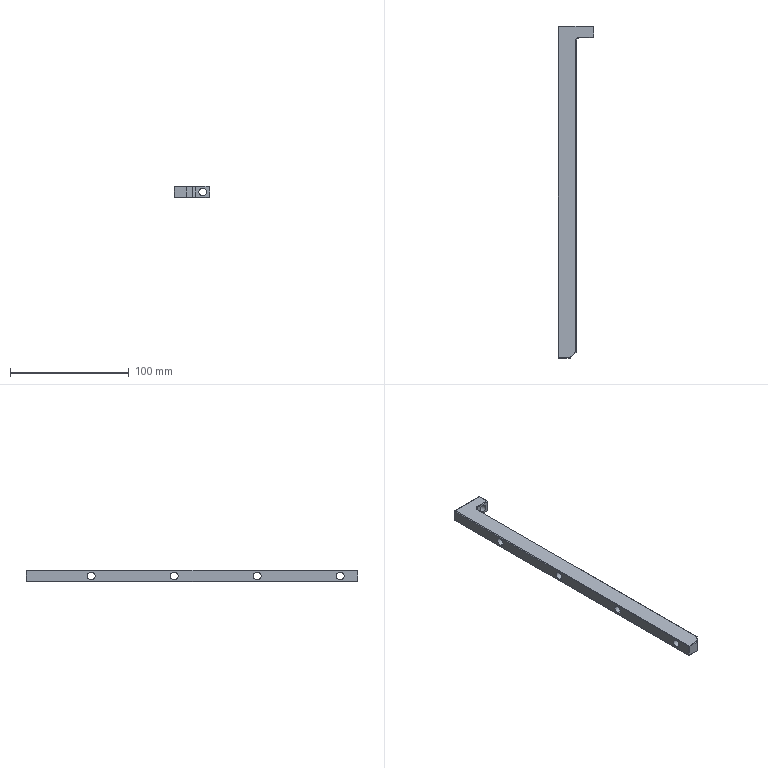Part | SolidWorks | features HoleWzd 3, Chamfer 2, Extrusion 1, Fillet 1, ICE 1 | 1 solid | 52 faces | box 30 x 280 x 10 mm | volume 40714 mm3 | plane 35 | cylinder 13 | cone 4 | commonest cylinder face diameters 6.6 x10 5 x2 6 x1
STEP:
#1=CARTESIAN_POINT('',(-9.,134.,-2.5));
#2=VERTEX_POINT('',#1);
#3=CARTESIAN_POINT('',(-9.,134.,2.5));
#4=VERTEX_POINT('',#3);
#5=CARTESIAN_POINT('',(-9.,134.,0.));
#6=DIRECTION('',(0.,1.,0.));
#7=DIRECTION('',(0.,0.,1.));
#8=AXIS2_PLACEMENT_3D('',#5,#6,#7);
#9=CIRCLE('',#8,2.5);
#10=EDGE_CURVE('',#2,#4,#9,.T.);
#11=ORIENTED_EDGE('',*,*,#10,.F.);
#12=CARTESIAN_POINT('',(-9.,140.,-2.5));
#13=VERTEX_POINT('',#12);
#14=CARTESIAN_POINT('',(-9.,140.,-2.5));
#15=DIRECTION('',(0.,1.,0.));
#16=VECTOR('',#15,1000.);
#17=LINE('',#14,#16);
#18=EDGE_CURVE('',#2,#13,#17,.T.);
#19=ORIENTED_EDGE('',*,*,#18,.T.);
#20=CARTESIAN_POINT('',(-9.,140.,2.5));
#21=VERTEX_POINT('',#20);
#22=CARTESIAN_POINT('',(-9.,140.,0.));
#23=DIRECTION('',(0.,1.,0.));
#24=DIRECTION('',(0.,0.,1.));
#25=AXIS2_PLACEMENT_3D('',#22,#23,#24);
#26=CIRCLE('',#25,2.5);
#27=EDGE_CURVE('',#13,#21,#26,.T.);
#28=ORIENTED_EDGE('',*,*,#27,.T.);
#29=CARTESIAN_POINT('',(-9.,140.,2.5));
#30=DIRECTION('',(0.,1.,0.));
#31=VECTOR('',#30,1000.);
#32=LINE('',#29,#31);
#33=EDGE_CURVE('',#4,#21,#32,.T.);
#34=ORIENTED_EDGE('',*,*,#33,.F.);
#35=EDGE_LOOP('',(#11,#19,#28,#34));
#36=FACE_OUTER_BOUND('',#35,.T.);
#37=CARTESIAN_POINT('',(-9.,140.,0.));
#38=DIRECTION('',(0.,1.,0.));
#39=DIRECTION('',(0.,0.,1.));
#40=AXIS2_PLACEMENT_3D('',#37,#38,#39);
#41=CYLINDRICAL_SURFACE('',#40,2.5);
#42=ADVANCED_FACE('',(#36),#41,.F.);
#43=CARTESIAN_POINT('',(-9.,132.498,0.));
#44=VERTEX_POINT('',#43);
#45=CARTESIAN_POINT('',(-9.,134.,2.5));
#46=DIRECTION('',(0.,0.515,0.8572));
#47=VECTOR('',#46,1000.);
#48=LINE('',#45,#47);
#49=EDGE_CURVE('',#44,#4,#48,.T.);
#50=ORIENTED_EDGE('',*,*,#49,.F.);
#51=CARTESIAN_POINT('',(-9.,134.,-2.5));
#52=DIRECTION('',(0.,0.515,-0.8572));
#53=VECTOR('',#52,1000.);
#54=LINE('',#51,#53);
#55=EDGE_CURVE('',#44,#2,#54,.T.);
#56=ORIENTED_EDGE('',*,*,#55,.T.);
#57=ORIENTED_EDGE('',*,*,#10,.T.);
#58=EDGE_LOOP('',(#50,#56,#57));
#59=FACE_OUTER_BOUND('',#58,.T.);
#60=CARTESIAN_POINT('',(-9.,134.,0.));
#61=DIRECTION('',(0.,1.,0.));
#62=DIRECTION('',(0.,0.,1.));
#63=AXIS2_PLACEMENT_3D('',#60,#61,#62);
#64=CONICAL_SURFACE('',#63,2.5,1.03);
#65=ADVANCED_FACE('',(#59),#64,.F.);
#66=CARTESIAN_POINT('',(-15.,85.,3.3));
#67=VERTEX_POINT('',#66);
#68=CARTESIAN_POINT('',(-15.,85.,-3.3));
#69=VERTEX_POINT('',#68);
#70=CARTESIAN_POINT('',(-15.,85.,0.));
#71=DIRECTION('',(1.,0.,0.));
#72=DIRECTION('',(0.,0.,-1.));
#73=AXIS2_PLACEMENT_3D('',#70,#71,#72);
#74=CIRCLE('',#73,3.3);
#75=EDGE_CURVE('',#67,#69,#74,.T.);
#76=ORIENTED_EDGE('',*,*,#75,.F.);
#77=CARTESIAN_POINT('',(0.,85.,3.3));
#78=VERTEX_POINT('',#77);
#79=CARTESIAN_POINT('',(0.,85.,3.3));
#80=DIRECTION('',(1.,0.,0.));
#81=VECTOR('',#80,1000.);
#82=LINE('',#79,#81);
#83=EDGE_CURVE('',#67,#78,#82,.T.);
#84=ORIENTED_EDGE('',*,*,#83,.T.);
#85=CARTESIAN_POINT('',(0.,85.,-3.3));
#86=VERTEX_POINT('',#85);
#87=CARTESIAN_POINT('',(0.,85.,0.));
#88=DIRECTION('',(1.,0.,0.));
#89=DIRECTION('',(0.,0.,-1.));
#90=AXIS2_PLACEMENT_3D('',#87,#88,#89);
#91=CIRCLE('',#90,3.3);
#92=EDGE_CURVE('',#78,#86,#91,.T.);
#93=ORIENTED_EDGE('',*,*,#92,.T.);
#94=CARTESIAN_POINT('',(0.,85.,-3.3));
#95=DIRECTION('',(1.,0.,0.));
#96=VECTOR('',#95,1000.);
#97=LINE('',#94,#96);
#98=EDGE_CURVE('',#69,#86,#97,.T.);
#99=ORIENTED_EDGE('',*,*,#98,.F.);
#100=EDGE_LOOP('',(#76,#84,#93,#99));
#101=FACE_OUTER_BOUND('',#100,.T.);
#102=CARTESIAN_POINT('',(0.,85.,0.));
#103=DIRECTION('',(1.,0.,0.));
#104=DIRECTION('',(0.,0.,-1.));
#105=AXIS2_PLACEMENT_3D('',#102,#103,#104);
#106=CYLINDRICAL_SURFACE('',#105,3.3);
#107=ADVANCED_FACE('',(#101),#106,.F.);
#108=CARTESIAN_POINT('',(-15.,15.,3.3));
#109=VERTEX_POINT('',#108);
#110=CARTESIAN_POINT('',(-15.,15.,-3.3));
#111=VERTEX_POINT('',#110);
#112=CARTESIAN_POINT('',(-15.,15.,0.));
#113=DIRECTION('',(1.,0.,0.));
#114=DIRECTION('',(0.,0.,-1.));
#115=AXIS2_PLACEMENT_3D('',#112,#113,#114);
#116=CIRCLE('',#115,3.3);
#117=EDGE_CURVE('',#109,#111,#116,.T.);
#118=ORIENTED_EDGE('',*,*,#117,.F.);
#119=CARTESIAN_POINT('',(0.,15.,3.3));
#120=VERTEX_POINT('',#119);
#121=CARTESIAN_POINT('',(0.,15.,3.3));
#122=DIRECTION('',(1.,0.,0.));
#123=VECTOR('',#122,1000.);
#124=LINE('',#121,#123);
#125=EDGE_CURVE('',#109,#120,#124,.T.);
#126=ORIENTED_EDGE('',*,*,#125,.T.);
#127=CARTESIAN_POINT('',(0.,15.,-3.3));
#128=VERTEX_POINT('',#127);
#129=CARTESIAN_POINT('',(0.,15.,0.));
#130=DIRECTION('',(1.,0.,0.));
#131=DIRECTION('',(0.,0.,-1.));
#132=AXIS2_PLACEMENT_3D('',#129,#130,#131);
#133=CIRCLE('',#132,3.3);
#134=EDGE_CURVE('',#120,#128,#133,.T.);
#135=ORIENTED_EDGE('',*,*,#134,.T.);
#136=CARTESIAN_POINT('',(0.,15.,-3.3));
#137=DIRECTION('',(1.,0.,0.));
#138=VECTOR('',#137,1000.);
#139=LINE('',#136,#138);
#140=EDGE_CURVE('',#111,#128,#139,.T.);
#141=ORIENTED_EDGE('',*,*,#140,.F.);
#142=EDGE_LOOP('',(#118,#126,#135,#141));
#143=FACE_OUTER_BOUND('',#142,.T.);
#144=CARTESIAN_POINT('',(0.,15.,0.));
#145=DIRECTION('',(1.,0.,0.));
#146=DIRECTION('',(0.,0.,-1.));
#147=AXIS2_PLACEMENT_3D('',#144,#145,#146);
#148=CYLINDRICAL_SURFACE('',#147,3.3);
#149=ADVANCED_FACE('',(#143),#148,.F.);
#150=CARTESIAN_POINT('',(-15.,-55.,3.3));
#151=VERTEX_POINT('',#150);
#152=CARTESIAN_POINT('',(-15.,-55.,-3.3));
#153=VERTEX_POINT('',#152);
#154=CARTESIAN_POINT('',(-15.,-55.,0.));
#155=DIRECTION('',(1.,0.,0.));
#156=DIRECTION('',(0.,0.,-1.));
#157=AXIS2_PLACEMENT_3D('',#154,#155,#156);
#158=CIRCLE('',#157,3.3);
#159=EDGE_CURVE('',#151,#153,#158,.T.);
#160=ORIENTED_EDGE('',*,*,#159,.F.);
#161=CARTESIAN_POINT('',(0.,-55.,3.3));
#162=VERTEX_POINT('',#161);
#163=CARTESIAN_POINT('',(0.,-55.,3.3));
#164=DIRECTION('',(1.,0.,0.));
#165=VECTOR('',#164,1000.);
#166=LINE('',#163,#165);
#167=EDGE_CURVE('',#151,#162,#166,.T.);
#168=ORIENTED_EDGE('',*,*,#167,.T.);
#169=CARTESIAN_POINT('',(0.,-55.,-3.3));
#170=VERTEX_POINT('',#169);
#171=CARTESIAN_POINT('',(0.,-55.,0.));
#172=DIRECTION('',(1.,0.,0.));
#173=DIRECTION('',(0.,0.,-1.));
#174=AXIS2_PLACEMENT_3D('',#171,#172,#173);
#175=CIRCLE('',#174,3.3);
#176=EDGE_CURVE('',#162,#170,#175,.T.);
#177=ORIENTED_EDGE('',*,*,#176,.T.);
#178=CARTESIAN_POINT('',(0.,-55.,-3.3));
#179=DIRECTION('',(1.,0.,0.));
#180=VECTOR('',#179,1000.);
#181=LINE('',#178,#180);
#182=EDGE_CURVE('',#153,#170,#181,.T.);
#183=ORIENTED_EDGE('',*,*,#182,.F.);
#184=EDGE_LOOP('',(#160,#168,#177,#183));
#185=FACE_OUTER_BOUND('',#184,.T.);
#186=CARTESIAN_POINT('',(0.,-55.,0.));
#187=DIRECTION('',(1.,0.,0.));
#188=DIRECTION('',(0.,0.,-1.));
#189=AXIS2_PLACEMENT_3D('',#186,#187,#188);
#190=CYLINDRICAL_SURFACE('',#189,3.3);
#191=ADVANCED_FACE('',(#185),#190,.F.);
#192=CARTESIAN_POINT('',(-15.,-125.,3.3));
#193=VERTEX_POINT('',#192);
#194=CARTESIAN_POINT('',(-15.,-125.,-3.3));
#195=VERTEX_POINT('',#194);
#196=CARTESIAN_POINT('',(-15.,-125.,0.));
#197=DIRECTION('',(1.,0.,0.));
#198=DIRECTION('',(0.,0.,-1.));
#199=AXIS2_PLACEMENT_3D('',#196,#197,#198);
#200=CIRCLE('',#199,3.3);
#201=EDGE_CURVE('',#193,#195,#200,.T.);
#202=ORIENTED_EDGE('',*,*,#201,.F.);
#203=CARTESIAN_POINT('',(0.,-125.,3.3));
#204=VERTEX_POINT('',#203);
#205=CARTESIAN_POINT('',(0.,-125.,3.3));
#206=DIRECTION('',(1.,0.,0.));
#207=VECTOR('',#206,1000.);
#208=LINE('',#205,#207);
#209=EDGE_CURVE('',#193,#204,#208,.T.);
#210=ORIENTED_EDGE('',*,*,#209,.T.);
#211=CARTESIAN_POINT('',(0.,-125.,-3.3));
#212=VERTEX_POINT('',#211);
#213=CARTESIAN_POINT('',(0.,-125.,0.));
#214=DIRECTION('',(1.,0.,0.));
#215=DIRECTION('',(0.,0.,-1.));
#216=AXIS2_PLACEMENT_3D('',#213,#214,#215);
#217=CIRCLE('',#216,3.3);
#218=EDGE_CURVE('',#204,#212,#217,.T.);
#219=ORIENTED_EDGE('',*,*,#218,.T.);
#220=CARTESIAN_POINT('',(0.,-125.,-3.3));
#221=DIRECTION('',(1.,0.,0.));
#222=VECTOR('',#221,1000.);
#223=LINE('',#220,#222);
#224=EDGE_CURVE('',#195,#212,#223,.T.);
#225=ORIENTED_EDGE('',*,*,#224,.F.);
#226=EDGE_LOOP('',(#202,#210,#219,#225));
#227=FACE_OUTER_BOUND('',#226,.T.);
#228=CARTESIAN_POINT('',(0.,-125.,0.));
#229=DIRECTION('',(1.,0.,0.));
#230=DIRECTION('',(0.,0.,-1.));
#231=AXIS2_PLACEMENT_3D('',#228,#229,#230);
#232=CYLINDRICAL_SURFACE('',#231,3.3);
#233=ADVANCED_FACE('',(#227),#232,.F.);
#234=CARTESIAN_POINT('',(9.,140.,3.3));
#235=VERTEX_POINT('',#234);
#236=CARTESIAN_POINT('',(9.,140.,-3.3));
#237=VERTEX_POINT('',#236);
#238=CARTESIAN_POINT('',(9.,140.,0.));
#239=DIRECTION('',(0.,-1.,0.));
#240=DIRECTION('',(0.,0.,-1.));
#241=AXIS2_PLACEMENT_3D('',#238,#239,#240);
#242=CIRCLE('',#241,3.3);
#243=EDGE_CURVE('',#235,#237,#242,.T.);
#244=ORIENTED_EDGE('',*,*,#243,.F.);
#245=CARTESIAN_POINT('',(9.,130.,3.3));
#246=VERTEX_POINT('',#245);
#247=CARTESIAN_POINT('',(9.,130.,3.3));
#248=DIRECTION('',(0.,-1.,0.));
#249=VECTOR('',#248,1000.);
#250=LINE('',#247,#249);
#251=EDGE_CURVE('',#235,#246,#250,.T.);
#252=ORIENTED_EDGE('',*,*,#251,.T.);
#253=CARTESIAN_POINT('',(9.,130.,-3.3));
#254=VERTEX_POINT('',#253);
#255=CARTESIAN_POINT('',(9.,130.,0.));
#256=DIRECTION('',(0.,-1.,0.));
#257=DIRECTION('',(0.,0.,-1.));
#258=AXIS2_PLACEMENT_3D('',#255,#256,#257);
#259=CIRCLE('',#258,3.3);
#260=EDGE_CURVE('',#246,#254,#259,.T.);
#261=ORIENTED_EDGE('',*,*,#260,.T.);
#262=CARTESIAN_POINT('',(9.,130.,-3.3));
#263=DIRECTION('',(0.,-1.,0.));
#264=VECTOR('',#263,1000.);
#265=LINE('',#262,#264);
#266=EDGE_CURVE('',#237,#254,#265,.T.);
#267=ORIENTED_EDGE('',*,*,#266,.F.);
#268=EDGE_LOOP('',(#244,#252,#261,#267));
#269=FACE_OUTER_BOUND('',#268,.T.);
#270=CARTESIAN_POINT('',(9.,130.,0.));
#271=DIRECTION('',(0.,-1.,0.));
#272=DIRECTION('',(0.,0.,-1.));
#273=AXIS2_PLACEMENT_3D('',#270,#271,#272);
#274=CYLINDRICAL_SURFACE('',#273,3.3);
#275=ADVANCED_FACE('',(#269),#274,.F.);
#276=CARTESIAN_POINT('',(15.,130.5,-4.5));
#277=VERTEX_POINT('',#276);
#278=CARTESIAN_POINT('',(15.,139.5,-4.5));
#279=VERTEX_POINT('',#278);
#280=CARTESIAN_POINT('',(15.,140.,-4.5));
#281=DIRECTION('',(0.,1.,0.));
#282=VECTOR('',#281,1000.);
#283=LINE('',#280,#282);
#284=EDGE_CURVE('',#277,#279,#283,.T.);
#285=ORIENTED_EDGE('',*,*,#284,.T.);
#286=CARTESIAN_POINT('',(15.,139.5,4.5));
#287=VERTEX_POINT('',#286);
#288=CARTESIAN_POINT('',(15.,139.5,5.));
#289=DIRECTION('',(0.,0.,1.));
#290=VECTOR('',#289,1000.);
#291=LINE('',#288,#290);
#292=EDGE_CURVE('',#279,#287,#291,.T.);
#293=ORIENTED_EDGE('',*,*,#292,.T.);
#294=CARTESIAN_POINT('',(15.,130.5,4.5));
#295=VERTEX_POINT('',#294);
#296=CARTESIAN_POINT('',(15.,-140.,4.5));
#297=DIRECTION('',(0.,-1.,0.));
#298=VECTOR('',#297,1000.);
#299=LINE('',#296,#298);
#300=EDGE_CURVE('',#287,#295,#299,.T.);
#301=ORIENTED_EDGE('',*,*,#300,.T.);
#302=CARTESIAN_POINT('',(15.,130.5,5.));
#303=DIRECTION('',(0.,0.,-1.));
#304=VECTOR('',#303,1000.);
#305=LINE('',#302,#304);
#306=EDGE_CURVE('',#295,#277,#305,.T.);
#307=ORIENTED_EDGE('',*,*,#306,.T.);
#308=EDGE_LOOP('',(#285,#293,#301,#307));
#309=FACE_OUTER_BOUND('',#308,.T.);
#310=CARTESIAN_POINT('',(15.,-140.,5.));
#311=DIRECTION('',(-1.,0.,0.));
#312=DIRECTION('',(0.,0.,1.));
#313=AXIS2_PLACEMENT_3D('',#310,#311,#312);
#314=PLANE('',#313);
#315=ADVANCED_FACE('',(#309),#314,.F.);
#316=CARTESIAN_POINT('',(-9.,140.,0.));
#317=DIRECTION('',(0.,1.,0.));
#318=DIRECTION('',(0.,0.,1.));
#319=AXIS2_PLACEMENT_3D('',#316,#317,#318);
#320=CIRCLE('',#319,2.5);
#321=EDGE_CURVE('',#21,#13,#320,.T.);
#322=ORIENTED_EDGE('',*,*,#321,.F.);
#323=ORIENTED_EDGE('',*,*,#27,.F.);
#324=EDGE_LOOP('',(#322,#323));
#325=FACE_BOUND('',#324,.T.);
#326=CARTESIAN_POINT('',(-14.5,140.,-4.5));
#327=VERTEX_POINT('',#326);
#328=CARTESIAN_POINT('',(-14.5,140.,4.5));
#329=VERTEX_POINT('',#328);
#330=CARTESIAN_POINT('',(-14.5,140.,5.));
#331=DIRECTION('',(0.,0.,1.));
#332=VECTOR('',#331,1000.);
#333=LINE('',#330,#332);
#334=EDGE_CURVE('',#327,#329,#333,.T.);
#335=ORIENTED_EDGE('',*,*,#334,.T.);
#336=CARTESIAN_POINT('',(14.5,140.,4.5));
#337=VERTEX_POINT('',#336);
#338=CARTESIAN_POINT('',(-15.,140.,4.5));
#339=DIRECTION('',(1.,0.,0.));
#340=VECTOR('',#339,1000.);
#341=LINE('',#338,#340);
#342=EDGE_CURVE('',#329,#337,#341,.T.);
#343=ORIENTED_EDGE('',*,*,#342,.T.);
#344=CARTESIAN_POINT('',(14.5,140.,-4.5));
#345=VERTEX_POINT('',#344);
#346=CARTESIAN_POINT('',(14.5,140.,5.));
#347=DIRECTION('',(0.,0.,-1.));
#348=VECTOR('',#347,1000.);
#349=LINE('',#346,#348);
#350=EDGE_CURVE('',#337,#345,#349,.T.);
#351=ORIENTED_EDGE('',*,*,#350,.T.);
#352=CARTESIAN_POINT('',(-15.,140.,-4.5));
#353=DIRECTION('',(-1.,0.,0.));
#354=VECTOR('',#353,1000.);
#355=LINE('',#352,#354);
#356=EDGE_CURVE('',#345,#327,#355,.T.);
#357=ORIENTED_EDGE('',*,*,#356,.T.);
#358=EDGE_LOOP('',(#335,#343,#351,#357));
#359=FACE_OUTER_BOUND('',#358,.T.);
#360=CARTESIAN_POINT('',(9.,140.,0.));
#361=DIRECTION('',(0.,-1.,0.));
#362=DIRECTION('',(0.,0.,-1.));
#363=AXIS2_PLACEMENT_3D('',#360,#361,#362);
#364=CIRCLE('',#363,3.3);
#365=EDGE_CURVE('',#237,#235,#364,.T.);
#366=ORIENTED_EDGE('',*,*,#365,.T.);
#367=ORIENTED_EDGE('',*,*,#243,.T.);
#368=EDGE_LOOP('',(#366,#367));
#369=FACE_BOUND('',#368,.T.);
#370=CARTESIAN_POINT('',(-15.,140.,5.));
#371=DIRECTION('',(0.,-1.,0.));
#372=DIRECTION('',(0.,0.,-1.));
#373=AXIS2_PLACEMENT_3D('',#370,#371,#372);
#374=PLANE('',#373);
#375=ADVANCED_FACE('',(#325,#359,#369),#374,.F.);
#376=CARTESIAN_POINT('',(-15.,-139.5,-4.5));
#377=VERTEX_POINT('',#376);
#378=CARTESIAN_POINT('',(-15.,-139.5,4.5));
#379=VERTEX_POINT('',#378);
#380=CARTESIAN_POINT('',(-15.,-139.5,5.));
#381=DIRECTION('',(0.,0.,1.));
#382=VECTOR('',#381,1000.);
#383=LINE('',#380,#382);
#384=EDGE_CURVE('',#377,#379,#383,.T.);
#385=ORIENTED_EDGE('',*,*,#384,.T.);
#386=CARTESIAN_POINT('',(-15.,139.5,4.5));
#387=VERTEX_POINT('',#386);
#388=CARTESIAN_POINT('',(-15.,-140.,4.5));
#389=DIRECTION('',(0.,1.,0.));
#390=VECTOR('',#389,1000.);
#391=LINE('',#388,#390);
#392=EDGE_CURVE('',#379,#387,#391,.T.);
#393=ORIENTED_EDGE('',*,*,#392,.T.);
#394=CARTESIAN_POINT('',(-15.,139.5,-4.5));
#395=VERTEX_POINT('',#394);
#396=CARTESIAN_POINT('',(-15.,139.5,5.));
#397=DIRECTION('',(0.,0.,-1.));
#398=VECTOR('',#397,1000.);
#399=LINE('',#396,#398);
#400=EDGE_CURVE('',#387,#395,#399,.T.);
#401=ORIENTED_EDGE('',*,*,#400,.T.);
#402=CARTESIAN_POINT('',(-15.,-140.,-4.5));
#403=DIRECTION('',(0.,-1.,0.));
#404=VECTOR('',#403,1000.);
#405=LINE('',#402,#404);
#406=EDGE_CURVE('',#395,#377,#405,.T.);
#407=ORIENTED_EDGE('',*,*,#406,.T.);
#408=EDGE_LOOP('',(#385,#393,#401,#407));
#409=FACE_OUTER_BOUND('',#408,.T.);
#410=CARTESIAN_POINT('',(-15.,85.,0.));
#411=DIRECTION('',(1.,0.,0.));
#412=DIRECTION('',(0.,0.,-1.));
#413=AXIS2_PLACEMENT_3D('',#410,#411,#412);
#414=CIRCLE('',#413,3.3);
#415=EDGE_CURVE('',#69,#67,#414,.T.);
#416=ORIENTED_EDGE('',*,*,#415,.T.);
#417=ORIENTED_EDGE('',*,*,#75,.T.);
#418=EDGE_LOOP('',(#416,#417));
#419=FACE_BOUND('',#418,.T.);
#420=CARTESIAN_POINT('',(-15.,15.,0.));
#421=DIRECTION('',(1.,0.,0.));
#422=DIRECTION('',(0.,0.,-1.));
#423=AXIS2_PLACEMENT_3D('',#420,#421,#422);
#424=CIRCLE('',#423,3.3);
#425=EDGE_CURVE('',#111,#109,#424,.T.);
#426=ORIENTED_EDGE('',*,*,#425,.T.);
#427=ORIENTED_EDGE('',*,*,#117,.T.);
#428=EDGE_LOOP('',(#426,#427));
#429=FACE_BOUND('',#428,.T.);
#430=CARTESIAN_POINT('',(-15.,-55.,0.));
#431=DIRECTION('',(1.,0.,0.));
#432=DIRECTION('',(0.,0.,-1.));
#433=AXIS2_PLACEMENT_3D('',#430,#431,#432);
#434=CIRCLE('',#433,3.3);
#435=EDGE_CURVE('',#153,#151,#434,.T.);
#436=ORIENTED_EDGE('',*,*,#435,.T.);
#437=ORIENTED_EDGE('',*,*,#159,.T.);
#438=EDGE_LOOP('',(#436,#437));
#439=FACE_BOUND('',#438,.T.);
#440=CARTESIAN_POINT('',(-15.,-125.,0.));
#441=DIRECTION('',(1.,0.,0.));
#442=DIRECTION('',(0.,0.,-1.));
#443=AXIS2_PLACEMENT_3D('',#440,#441,#442);
#444=CIRCLE('',#443,3.3);
#445=EDGE_CURVE('',#195,#193,#444,.T.);
#446=ORIENTED_EDGE('',*,*,#445,.T.);
#447=ORIENTED_EDGE('',*,*,#201,.T.);
#448=EDGE_LOOP('',(#446,#447));
#449=FACE_BOUND('',#448,.T.);
#450=CARTESIAN_POINT('',(-15.,-140.,5.));
#451=DIRECTION('',(1.,0.,0.));
#452=DIRECTION('',(0.,0.,-1.));
#453=AXIS2_PLACEMENT_3D('',#450,#451,#452);
#454=PLANE('',#453);
#455=ADVANCED_FACE('',(#409,#419,#429,#439,#449),#454,.F.);
#456=CARTESIAN_POINT('',(-5.,-140.,-4.5));
#457=VERTEX_POINT('',#456);
#458=CARTESIAN_POINT('',(-5.,-140.,4.5));
#459=VERTEX_POINT('',#458);
#460=CARTESIAN_POINT('',(-5.,-140.,5.));
#461=DIRECTION('',(0.,0.,1.));
#462=VECTOR('',#461,1000.);
#463=LINE('',#460,#462);
#464=EDGE_CURVE('',#457,#459,#463,.T.);
#465=ORIENTED_EDGE('',*,*,#464,.T.);
#466=CARTESIAN_POINT('',(-14.5,-140.,4.5));
#467=VERTEX_POINT('',#466);
#468=CARTESIAN_POINT('',(-15.,-140.,4.5));
#469=DIRECTION('',(-1.,0.,0.));
#470=VECTOR('',#469,1000.);
#471=LINE('',#468,#470);
#472=EDGE_CURVE('',#459,#467,#471,.T.);
#473=ORIENTED_EDGE('',*,*,#472,.T.);
#474=CARTESIAN_POINT('',(-14.5,-140.,-4.5));
#475=VERTEX_POINT('',#474);
#476=CARTESIAN_POINT('',(-14.5,-140.,5.));
#477=DIRECTION('',(0.,0.,-1.));
#478=VECTOR('',#477,1000.);
#479=LINE('',#476,#478);
#480=EDGE_CURVE('',#467,#475,#479,.T.);
#481=ORIENTED_EDGE('',*,*,#480,.T.);
#482=CARTESIAN_POINT('',(-5.,-140.,-4.5));
#483=DIRECTION('',(1.,0.,0.));
#484=VECTOR('',#483,1000.);
#485=LINE('',#482,#484);
#486=EDGE_CURVE('',#475,#457,#485,.T.);
#487=ORIENTED_EDGE('',*,*,#486,.T.);
#488=EDGE_LOOP('',(#465,#473,#481,#487));
#489=FACE_OUTER_BOUND('',#488,.T.);
#490=CARTESIAN_POINT('',(-15.,-140.,5.));
#491=DIRECTION('',(0.,1.,0.));
#492=DIRECTION('',(0.,0.,1.));
#493=AXIS2_PLACEMENT_3D('',#490,#491,#492);
#494=PLANE('',#493);
#495=ADVANCED_FACE('',(#489),#494,.F.);
#496=CARTESIAN_POINT('',(-0.5,-134.793,5.));
#497=VERTEX_POINT('',#496);
#498=CARTESIAN_POINT('',(-0.5,127.,5.));
#499=VERTEX_POINT('',#498);
#500=CARTESIAN_POINT('',(-0.5,0.,5.));
#501=DIRECTION('',(0.,1.,0.));
#502=VECTOR('',#501,1000.);
#503=LINE('',#500,#502);
#504=EDGE_CURVE('',#497,#499,#503,.T.);
#505=ORIENTED_EDGE('',*,*,#504,.T.);
#506=CARTESIAN_POINT('',(3.,130.5,5.));
#507=VERTEX_POINT('',#506);
#508=CARTESIAN_POINT('',(3.,127.,5.));
#509=DIRECTION('',(0.,0.,-1.));
#510=DIRECTION('',(-1.,0.,0.));
#511=AXIS2_PLACEMENT_3D('',#508,#509,#510);
#512=CIRCLE('',#511,3.5);
#513=EDGE_CURVE('',#499,#507,#512,.T.);
#514=ORIENTED_EDGE('',*,*,#513,.T.);
#515=CARTESIAN_POINT('',(14.5,130.5,5.));
#516=VERTEX_POINT('',#515);
#517=CARTESIAN_POINT('',(0.,130.5,5.));
#518=DIRECTION('',(1.,0.,0.));
#519=VECTOR('',#518,1000.);
#520=LINE('',#517,#519);
#521=EDGE_CURVE('',#507,#516,#520,.T.);
#522=ORIENTED_EDGE('',*,*,#521,.T.);
#523=CARTESIAN_POINT('',(14.5,139.5,5.));
#524=VERTEX_POINT('',#523);
#525=CARTESIAN_POINT('',(14.5,0.,5.));
#526=DIRECTION('',(0.,1.,0.));
#527=VECTOR('',#526,1000.);
#528=LINE('',#525,#527);
#529=EDGE_CURVE('',#516,#524,#528,.T.);
#530=ORIENTED_EDGE('',*,*,#529,.T.);
#531=CARTESIAN_POINT('',(-14.5,139.5,5.));
#532=VERTEX_POINT('',#531);
#533=CARTESIAN_POINT('',(0.,139.5,5.));
#534=DIRECTION('',(-1.,0.,0.));
#535=VECTOR('',#534,1000.);
#536=LINE('',#533,#535);
#537=EDGE_CURVE('',#524,#532,#536,.T.);
#538=ORIENTED_EDGE('',*,*,#537,.T.);
#539=CARTESIAN_POINT('',(-14.5,-139.5,5.));
#540=VERTEX_POINT('',#539);
#541=CARTESIAN_POINT('',(-14.5,0.,5.));
#542=DIRECTION('',(0.,-1.,0.));
#543=VECTOR('',#542,1000.);
#544=LINE('',#541,#543);
#545=EDGE_CURVE('',#532,#540,#544,.T.);
#546=ORIENTED_EDGE('',*,*,#545,.T.);
#547=CARTESIAN_POINT('',(-5.207,-139.5,5.));
#548=VERTEX_POINT('',#547);
#549=CARTESIAN_POINT('',(0.,-139.5,5.));
#550=DIRECTION('',(1.,0.,0.));
#551=VECTOR('',#550,1000.);
#552=LINE('',#549,#551);
#553=EDGE_CURVE('',#540,#548,#552,.T.);
#554=ORIENTED_EDGE('',*,*,#553,.T.);
#555=CARTESIAN_POINT('',(-0.3536,-134.646,5.));
#556=DIRECTION('',(0.7071,0.7071,0.));
#557=VECTOR('',#556,1000.);
#558=LINE('',#555,#557);
#559=EDGE_CURVE('',#548,#497,#558,.T.);
#560=ORIENTED_EDGE('',*,*,#559,.T.);
#561=EDGE_LOOP('',(#505,#514,#522,#530,#538,#546,#554,#560));
#562=FACE_OUTER_BOUND('',#561,.T.);
#563=CARTESIAN_POINT('',(0.,0.,5.));
#564=DIRECTION('',(0.,0.,-1.));
#565=DIRECTION('',(-1.,0.,0.));
#566=AXIS2_PLACEMENT_3D('',#563,#564,#565);
#567=PLANE('',#566);
#568=ADVANCED_FACE('',(#562),#567,.F.);
#569=CARTESIAN_POINT('',(14.5,130.5,-5.));
#570=VERTEX_POINT('',#569);
#571=CARTESIAN_POINT('',(3.,130.5,-5.));
#572=VERTEX_POINT('',#571);
#573=CARTESIAN_POINT('',(3.,130.5,-5.));
#574=DIRECTION('',(-1.,0.,0.));
#575=VECTOR('',#574,1000.);
#576=LINE('',#573,#575);
#577=EDGE_CURVE('',#570,#572,#576,.T.);
#578=ORIENTED_EDGE('',*,*,#577,.T.);
#579=CARTESIAN_POINT('',(-0.5,127.,-5.));
#580=VERTEX_POINT('',#579);
#581=CARTESIAN_POINT('',(3.,127.,-5.));
#582=DIRECTION('',(0.,0.,1.));
#583=DIRECTION('',(-1.,0.,0.));
#584=AXIS2_PLACEMENT_3D('',#581,#582,#583);
#585=CIRCLE('',#584,3.5);
#586=EDGE_CURVE('',#572,#580,#585,.T.);
#587=ORIENTED_EDGE('',*,*,#586,.T.);
#588=CARTESIAN_POINT('',(-0.5,-134.793,-5.));
#589=VERTEX_POINT('',#588);
#590=CARTESIAN_POINT('',(-0.5,-135.,-5.));
#591=DIRECTION('',(0.,-1.,0.));
#592=VECTOR('',#591,1000.);
#593=LINE('',#590,#592);
#594=EDGE_CURVE('',#580,#589,#593,.T.);
#595=ORIENTED_EDGE('',*,*,#594,.T.);
#596=CARTESIAN_POINT('',(-5.207,-139.5,-5.));
#597=VERTEX_POINT('',#596);
#598=CARTESIAN_POINT('',(67.146,-67.146,-5.));
#599=DIRECTION('',(-0.7071,-0.7071,0.));
#600=VECTOR('',#599,1000.);
#601=LINE('',#598,#600);
#602=EDGE_CURVE('',#589,#597,#601,.T.);
#603=ORIENTED_EDGE('',*,*,#602,.T.);
#604=CARTESIAN_POINT('',(-14.5,-139.5,-5.));
#605=VERTEX_POINT('',#604);
#606=CARTESIAN_POINT('',(-15.,-139.5,-5.));
#607=DIRECTION('',(-1.,0.,0.));
#608=VECTOR('',#607,1000.);
#609=LINE('',#606,#608);
#610=EDGE_CURVE('',#597,#605,#609,.T.);
#611=ORIENTED_EDGE('',*,*,#610,.T.);
#612=CARTESIAN_POINT('',(-14.5,139.5,-5.));
#613=VERTEX_POINT('',#612);
#614=CARTESIAN_POINT('',(-14.5,140.,-5.));
#615=DIRECTION('',(0.,1.,0.));
#616=VECTOR('',#615,1000.);
#617=LINE('',#614,#616);
#618=EDGE_CURVE('',#605,#613,#617,.T.);
#619=ORIENTED_EDGE('',*,*,#618,.T.);
#620=CARTESIAN_POINT('',(14.5,139.5,-5.));
#621=VERTEX_POINT('',#620);
#622=CARTESIAN_POINT('',(15.,139.5,-5.));
#623=DIRECTION('',(1.,0.,0.));
#624=VECTOR('',#623,1000.);
#625=LINE('',#622,#624);
#626=EDGE_CURVE('',#613,#621,#625,.T.);
#627=ORIENTED_EDGE('',*,*,#626,.T.);
#628=CARTESIAN_POINT('',(14.5,130.,-5.));
#629=DIRECTION('',(0.,-1.,0.));
#630=VECTOR('',#629,1000.);
#631=LINE('',#628,#630);
#632=EDGE_CURVE('',#621,#570,#631,.T.);
#633=ORIENTED_EDGE('',*,*,#632,.T.);
#634=EDGE_LOOP('',(#578,#587,#595,#603,#611,#619,#627,#633));
#635=FACE_OUTER_BOUND('',#634,.T.);
#636=CARTESIAN_POINT('',(0.,0.,-5.));
#637=DIRECTION('',(0.,0.,-1.));
#638=DIRECTION('',(-1.,0.,0.));
#639=AXIS2_PLACEMENT_3D('',#636,#637,#638);
#640=PLANE('',#639);
#641=ADVANCED_FACE('',(#635),#640,.T.);
#642=CARTESIAN_POINT('',(9.,130.,0.));
#643=DIRECTION('',(0.,-1.,0.));
#644=DIRECTION('',(0.,0.,-1.));
#645=AXIS2_PLACEMENT_3D('',#642,#643,#644);
#646=CIRCLE('',#645,3.3);
#647=EDGE_CURVE('',#254,#246,#646,.T.);
#648=ORIENTED_EDGE('',*,*,#647,.F.);
#649=ORIENTED_EDGE('',*,*,#260,.F.);
#650=EDGE_LOOP('',(#648,#649));
#651=FACE_BOUND('',#650,.T.);
#652=CARTESIAN_POINT('',(14.5,130.,-4.5));
#653=VERTEX_POINT('',#652);
#654=CARTESIAN_POINT('',(14.5,130.,4.5));
#655=VERTEX_POINT('',#654);
#656=CARTESIAN_POINT('',(14.5,130.,5.));
#657=DIRECTION('',(0.,0.,1.));
#658=VECTOR('',#657,1000.);
#659=LINE('',#656,#658);
#660=EDGE_CURVE('',#653,#655,#659,.T.);
#661=ORIENTED_EDGE('',*,*,#660,.T.);
#662=CARTESIAN_POINT('',(3.,130.,4.5));
#663=VERTEX_POINT('',#662);
#664=CARTESIAN_POINT('',(15.,130.,4.5));
#665=DIRECTION('',(-1.,0.,0.));
#666=VECTOR('',#665,1000.);
#667=LINE('',#664,#666);
#668=EDGE_CURVE('',#655,#663,#667,.T.);
#669=ORIENTED_EDGE('',*,*,#668,.T.);
#670=CARTESIAN_POINT('',(3.,130.,-4.5));
#671=VERTEX_POINT('',#670);
#672=CARTESIAN_POINT('',(3.,130.,-5.));
#673=DIRECTION('',(0.,0.,-1.));
#674=VECTOR('',#673,1000.);
#675=LINE('',#672,#674);
#676=EDGE_CURVE('',#663,#671,#675,.T.);
#677=ORIENTED_EDGE('',*,*,#676,.T.);
#678=CARTESIAN_POINT('',(15.,130.,-4.5));
#679=DIRECTION('',(1.,0.,0.));
#680=VECTOR('',#679,1000.);
#681=LINE('',#678,#680);
#682=EDGE_CURVE('',#671,#653,#681,.T.);
#683=ORIENTED_EDGE('',*,*,#682,.T.);
#684=EDGE_LOOP('',(#661,#669,#677,#683));
#685=FACE_OUTER_BOUND('',#684,.T.);
#686=CARTESIAN_POINT('',(15.,130.,5.));
#687=DIRECTION('',(0.,1.,0.));
#688=DIRECTION('',(0.,0.,1.));
#689=AXIS2_PLACEMENT_3D('',#686,#687,#688);
#690=PLANE('',#689);
#691=ADVANCED_FACE('',(#651,#685),#690,.F.);
#692=CARTESIAN_POINT('',(0.,85.,0.));
#693=DIRECTION('',(1.,0.,0.));
#694=DIRECTION('',(0.,0.,-1.));
#695=AXIS2_PLACEMENT_3D('',#692,#693,#694);
#696=CIRCLE('',#695,3.3);
#697=EDGE_CURVE('',#86,#78,#696,.T.);
#698=ORIENTED_EDGE('',*,*,#697,.F.);
#699=ORIENTED_EDGE('',*,*,#92,.F.);
#700=EDGE_LOOP('',(#698,#699));
#701=FACE_BOUND('',#700,.T.);
#702=CARTESIAN_POINT('',(0.,15.,0.));
#703=DIRECTION('',(1.,0.,0.));
#704=DIRECTION('',(0.,0.,-1.));
#705=AXIS2_PLACEMENT_3D('',#702,#703,#704);
#706=CIRCLE('',#705,3.3);
#707=EDGE_CURVE('',#128,#120,#706,.T.);
#708=ORIENTED_EDGE('',*,*,#707,.F.);
#709=ORIENTED_EDGE('',*,*,#134,.F.);
#710=EDGE_LOOP('',(#708,#709));
#711=FACE_BOUND('',#710,.T.);
#712=CARTESIAN_POINT('',(0.,-55.,0.));
#713=DIRECTION('',(1.,0.,0.));
#714=DIRECTION('',(0.,0.,-1.));
#715=AXIS2_PLACEMENT_3D('',#712,#713,#714);
#716=CIRCLE('',#715,3.3);
#717=EDGE_CURVE('',#170,#162,#716,.T.);
#718=ORIENTED_EDGE('',*,*,#717,.F.);
#719=ORIENTED_EDGE('',*,*,#176,.F.);
#720=EDGE_LOOP('',(#718,#719));
#721=FACE_BOUND('',#720,.T.);
#722=CARTESIAN_POINT('',(0.,-125.,0.));
#723=DIRECTION('',(1.,0.,0.));
#724=DIRECTION('',(0.,0.,-1.));
#725=AXIS2_PLACEMENT_3D('',#722,#723,#724);
#726=CIRCLE('',#725,3.3);
#727=EDGE_CURVE('',#212,#204,#726,.T.);
#728=ORIENTED_EDGE('',*,*,#727,.F.);
#729=ORIENTED_EDGE('',*,*,#218,.F.);
#730=EDGE_LOOP('',(#728,#729));
#731=FACE_BOUND('',#730,.T.);
#732=CARTESIAN_POINT('',(0.,127.,-4.5));
#733=VERTEX_POINT('',#732);
#734=CARTESIAN_POINT('',(0.,127.,4.5));
#735=VERTEX_POINT('',#734);
#736=CARTESIAN_POINT('',(0.,127.,5.));
#737=DIRECTION('',(0.,0.,1.));
#738=VECTOR('',#737,1000.);
#739=LINE('',#736,#738);
#740=EDGE_CURVE('',#733,#735,#739,.T.);
#741=ORIENTED_EDGE('',*,*,#740,.T.);
#742=CARTESIAN_POINT('',(0.,-135.,4.5));
#743=VERTEX_POINT('',#742);
#744=CARTESIAN_POINT('',(0.,-140.,4.5));
#745=DIRECTION('',(0.,-1.,0.));
#746=VECTOR('',#745,1000.);
#747=LINE('',#744,#746);
#748=EDGE_CURVE('',#735,#743,#747,.T.);
#749=ORIENTED_EDGE('',*,*,#748,.T.);
#750=CARTESIAN_POINT('',(0.,-135.,-4.5));
#751=VERTEX_POINT('',#750);
#752=CARTESIAN_POINT('',(0.,-135.,5.));
#753=DIRECTION('',(0.,0.,-1.));
#754=VECTOR('',#753,1000.);
#755=LINE('',#752,#754);
#756=EDGE_CURVE('',#743,#751,#755,.T.);
#757=ORIENTED_EDGE('',*,*,#756,.T.);
#758=CARTESIAN_POINT('',(0.,127.,-4.5));
#759=DIRECTION('',(0.,1.,0.));
#760=VECTOR('',#759,1000.);
#761=LINE('',#758,#760);
#762=EDGE_CURVE('',#751,#733,#761,.T.);
#763=ORIENTED_EDGE('',*,*,#762,.T.);
#764=EDGE_LOOP('',(#741,#749,#757,#763));
#765=FACE_OUTER_BOUND('',#764,.T.);
#766=CARTESIAN_POINT('',(0.,-140.,5.));
#767=DIRECTION('',(-1.,0.,0.));
#768=DIRECTION('',(0.,0.,1.));
#769=AXIS2_PLACEMENT_3D('',#766,#767,#768);
#770=PLANE('',#769);
#771=ADVANCED_FACE('',(#701,#711,#721,#731,#765),#770,.F.);
#772=ORIENTED_EDGE('',*,*,#676,.F.);
#773=CARTESIAN_POINT('',(3.,127.,4.5));
#774=DIRECTION('',(0.,0.,1.));
#775=DIRECTION('',(-1.,0.,0.));
#776=AXIS2_PLACEMENT_3D('',#773,#774,#775);
#777=CIRCLE('',#776,3.);
#778=EDGE_CURVE('',#663,#735,#777,.T.);
#779=ORIENTED_EDGE('',*,*,#778,.T.);
#780=ORIENTED_EDGE('',*,*,#740,.F.);
#781=CARTESIAN_POINT('',(3.,127.,-4.5));
#782=DIRECTION('',(0.,0.,-1.));
#783=DIRECTION('',(-1.,0.,0.));
#784=AXIS2_PLACEMENT_3D('',#781,#782,#783);
#785=CIRCLE('',#784,3.);
#786=EDGE_CURVE('',#733,#671,#785,.T.);
#787=ORIENTED_EDGE('',*,*,#786,.T.);
#788=EDGE_LOOP('',(#772,#779,#780,#787));
#789=FACE_OUTER_BOUND('',#788,.T.);
#790=CARTESIAN_POINT('',(3.,127.,5.));
#791=DIRECTION('',(0.,0.,1.));
#792=DIRECTION('',(1.,0.,0.));
#793=AXIS2_PLACEMENT_3D('',#790,#791,#792);
#794=CYLINDRICAL_SURFACE('',#793,3.);
#795=ADVANCED_FACE('',(#789),#794,.F.);
#796=ORIENTED_EDGE('',*,*,#251,.F.);
#797=ORIENTED_EDGE('',*,*,#365,.F.);
#798=ORIENTED_EDGE('',*,*,#266,.T.);
#799=ORIENTED_EDGE('',*,*,#647,.T.);
#800=EDGE_LOOP('',(#796,#797,#798,#799));
#801=FACE_OUTER_BOUND('',#800,.T.);
#802=CARTESIAN_POINT('',(9.,130.,0.));
#803=DIRECTION('',(0.,-1.,0.));
#804=DIRECTION('',(0.,0.,-1.));
#805=AXIS2_PLACEMENT_3D('',#802,#803,#804);
#806=CYLINDRICAL_SURFACE('',#805,3.3);
#807=ADVANCED_FACE('',(#801),#806,.F.);
#808=ORIENTED_EDGE('',*,*,#756,.F.);
#809=CARTESIAN_POINT('',(-5.,-140.,4.5));
#810=DIRECTION('',(-0.7071,-0.7071,0.));
#811=VECTOR('',#810,1000.);
#812=LINE('',#809,#811);
#813=EDGE_CURVE('',#743,#459,#812,.T.);
#814=ORIENTED_EDGE('',*,*,#813,.T.);
#815=ORIENTED_EDGE('',*,*,#464,.F.);
#816=CARTESIAN_POINT('',(0.,-135.,-4.5));
#817=DIRECTION('',(0.7071,0.7071,0.));
#818=VECTOR('',#817,1000.);
#819=LINE('',#816,#818);
#820=EDGE_CURVE('',#457,#751,#819,.T.);
#821=ORIENTED_EDGE('',*,*,#820,.T.);
#822=EDGE_LOOP('',(#808,#814,#815,#821));
#823=FACE_OUTER_BOUND('',#822,.T.);
#824=CARTESIAN_POINT('',(0.,-135.,5.));
#825=DIRECTION('',(-0.7071,0.7071,0.));
#826=DIRECTION('',(0.,0.,-1.));
#827=AXIS2_PLACEMENT_3D('',#824,#825,#826);
#828=PLANE('',#827);
#829=ADVANCED_FACE('',(#823),#828,.F.);
#830=ORIENTED_EDGE('',*,*,#209,.F.);
#831=ORIENTED_EDGE('',*,*,#445,.F.);
#832=ORIENTED_EDGE('',*,*,#224,.T.);
#833=ORIENTED_EDGE('',*,*,#727,.T.);
#834=EDGE_LOOP('',(#830,#831,#832,#833));
#835=FACE_OUTER_BOUND('',#834,.T.);
#836=CARTESIAN_POINT('',(0.,-125.,0.));
#837=DIRECTION('',(1.,0.,0.));
#838=DIRECTION('',(0.,0.,-1.));
#839=AXIS2_PLACEMENT_3D('',#836,#837,#838);
#840=CYLINDRICAL_SURFACE('',#839,3.3);
#841=ADVANCED_FACE('',(#835),#840,.F.);
#842=ORIENTED_EDGE('',*,*,#167,.F.);
#843=ORIENTED_EDGE('',*,*,#435,.F.);
#844=ORIENTED_EDGE('',*,*,#182,.T.);
#845=ORIENTED_EDGE('',*,*,#717,.T.);
#846=EDGE_LOOP('',(#842,#843,#844,#845));
#847=FACE_OUTER_BOUND('',#846,.T.);
#848=CARTESIAN_POINT('',(0.,-55.,0.));
#849=DIRECTION('',(1.,0.,0.));
#850=DIRECTION('',(0.,0.,-1.));
#851=AXIS2_PLACEMENT_3D('',#848,#849,#850);
#852=CYLINDRICAL_SURFACE('',#851,3.3);
#853=ADVANCED_FACE('',(#847),#852,.F.);
#854=ORIENTED_EDGE('',*,*,#125,.F.);
#855=ORIENTED_EDGE('',*,*,#425,.F.);
#856=ORIENTED_EDGE('',*,*,#140,.T.);
#857=ORIENTED_EDGE('',*,*,#707,.T.);
#858=EDGE_LOOP('',(#854,#855,#856,#857));
#859=FACE_OUTER_BOUND('',#858,.T.);
#860=CARTESIAN_POINT('',(0.,15.,0.));
#861=DIRECTION('',(1.,0.,0.));
#862=DIRECTION('',(0.,0.,-1.));
#863=AXIS2_PLACEMENT_3D('',#860,#861,#862);
#864=CYLINDRICAL_SURFACE('',#863,3.3);
#865=ADVANCED_FACE('',(#859),#864,.F.);
#866=ORIENTED_EDGE('',*,*,#83,.F.);
#867=ORIENTED_EDGE('',*,*,#415,.F.);
#868=ORIENTED_EDGE('',*,*,#98,.T.);
#869=ORIENTED_EDGE('',*,*,#697,.T.);
#870=EDGE_LOOP('',(#866,#867,#868,#869));
#871=FACE_OUTER_BOUND('',#870,.T.);
#872=CARTESIAN_POINT('',(0.,85.,0.));
#873=DIRECTION('',(1.,0.,0.));
#874=DIRECTION('',(0.,0.,-1.));
#875=AXIS2_PLACEMENT_3D('',#872,#873,#874);
#876=CYLINDRICAL_SURFACE('',#875,3.3);
#877=ADVANCED_FACE('',(#871),#876,.F.);
#878=CARTESIAN_POINT('',(14.5,130.,-4.5));
#879=DIRECTION('',(0.,0.7071,-0.7071));
#880=VECTOR('',#879,1000.);
#881=LINE('',#878,#880);
#882=EDGE_CURVE('',#653,#570,#881,.T.);
#883=ORIENTED_EDGE('',*,*,#882,.F.);
#884=ORIENTED_EDGE('',*,*,#682,.F.);
#885=CARTESIAN_POINT('',(3.,130.5,-5.));
#886=DIRECTION('',(0.,-0.7071,0.7071));
#887=VECTOR('',#886,1000.);
#888=LINE('',#885,#887);
#889=EDGE_CURVE('',#572,#671,#888,.T.);
#890=ORIENTED_EDGE('',*,*,#889,.F.);
#891=ORIENTED_EDGE('',*,*,#577,.F.);
#892=EDGE_LOOP('',(#883,#884,#890,#891));
#893=FACE_OUTER_BOUND('',#892,.T.);
#894=CARTESIAN_POINT('',(15.,130.,-4.5));
#895=DIRECTION('',(0.,-0.7071,-0.7071));
#896=DIRECTION('',(-1.,0.,0.));
#897=AXIS2_PLACEMENT_3D('',#894,#895,#896);
#898=PLANE('',#897);
#899=ADVANCED_FACE('',(#893),#898,.T.);
#900=CARTESIAN_POINT('',(14.5,130.,-4.5));
#901=DIRECTION('',(0.7071,0.7071,0.));
#902=VECTOR('',#901,1000.);
#903=LINE('',#900,#902);
#904=EDGE_CURVE('',#653,#277,#903,.T.);
#905=ORIENTED_EDGE('',*,*,#904,.F.);
#906=ORIENTED_EDGE('',*,*,#882,.T.);
#907=CARTESIAN_POINT('',(14.75,130.5,-4.75));
#908=DIRECTION('',(-0.7071,0.,-0.7071));
#909=VECTOR('',#908,1000.);
#910=LINE('',#907,#909);
#911=EDGE_CURVE('',#277,#570,#910,.T.);
#912=ORIENTED_EDGE('',*,*,#911,.F.);
#913=EDGE_LOOP('',(#905,#906,#912));
#914=FACE_OUTER_BOUND('',#913,.T.);
#915=CARTESIAN_POINT('',(14.5,130.,-4.5));
#916=DIRECTION('',(0.5774,-0.5774,-0.5774));
#917=DIRECTION('',(0.,0.7071,-0.7071));
#918=AXIS2_PLACEMENT_3D('',#915,#916,#917);
#919=PLANE('',#918);
#920=ADVANCED_FACE('',(#914),#919,.T.);
#921=ORIENTED_EDGE('',*,*,#889,.T.);
#922=ORIENTED_EDGE('',*,*,#786,.F.);
#923=CARTESIAN_POINT('',(-0.5,127.,-5.));
#924=DIRECTION('',(0.7071,0.,0.7071));
#925=VECTOR('',#924,1000.);
#926=LINE('',#923,#925);
#927=EDGE_CURVE('',#580,#733,#926,.T.);
#928=ORIENTED_EDGE('',*,*,#927,.F.);
#929=ORIENTED_EDGE('',*,*,#586,.F.);
#930=EDGE_LOOP('',(#921,#922,#928,#929));
#931=FACE_OUTER_BOUND('',#930,.T.);
#932=CARTESIAN_POINT('',(3.,127.,-5.));
#933=DIRECTION('',(0.,0.,-1.));
#934=DIRECTION('',(-1.,0.,0.));
#935=AXIS2_PLACEMENT_3D('',#932,#933,#934);
#936=CONICAL_SURFACE('',#935,3.5,0.7854);
#937=ADVANCED_FACE('',(#931),#936,.F.);
#938=ORIENTED_EDGE('',*,*,#911,.T.);
#939=ORIENTED_EDGE('',*,*,#632,.F.);
#940=CARTESIAN_POINT('',(14.75,139.5,-4.75));
#941=DIRECTION('',(-0.7071,0.,-0.7071));
#942=VECTOR('',#941,1000.);
#943=LINE('',#940,#942);
#944=EDGE_CURVE('',#279,#621,#943,.T.);
#945=ORIENTED_EDGE('',*,*,#944,.F.);
#946=ORIENTED_EDGE('',*,*,#284,.F.);
#947=EDGE_LOOP('',(#938,#939,#945,#946));
#948=FACE_OUTER_BOUND('',#947,.T.);
#949=CARTESIAN_POINT('',(15.,-140.,-4.5));
#950=DIRECTION('',(0.7071,0.,-0.7071));
#951=DIRECTION('',(0.,-1.,0.));
#952=AXIS2_PLACEMENT_3D('',#949,#950,#951);
#953=PLANE('',#952);
#954=ADVANCED_FACE('',(#948),#953,.T.);
#955=ORIENTED_EDGE('',*,*,#904,.T.);
#956=ORIENTED_EDGE('',*,*,#306,.F.);
#957=CARTESIAN_POINT('',(14.75,130.25,4.5));
#958=DIRECTION('',(0.7071,0.7071,0.));
#959=VECTOR('',#958,1000.);
#960=LINE('',#957,#959);
#961=EDGE_CURVE('',#655,#295,#960,.T.);
#962=ORIENTED_EDGE('',*,*,#961,.F.);
#963=ORIENTED_EDGE('',*,*,#660,.F.);
#964=EDGE_LOOP('',(#955,#956,#962,#963));
#965=FACE_OUTER_BOUND('',#964,.T.);
#966=CARTESIAN_POINT('',(15.,130.5,5.));
#967=DIRECTION('',(-0.7071,0.7071,0.));
#968=DIRECTION('',(0.,0.,-1.));
#969=AXIS2_PLACEMENT_3D('',#966,#967,#968);
#970=PLANE('',#969);
#971=ADVANCED_FACE('',(#965),#970,.F.);
#972=CARTESIAN_POINT('',(3.,130.,4.5));
#973=DIRECTION('',(0.,0.7071,0.7071));
#974=VECTOR('',#973,1000.);
#975=LINE('',#972,#974);
#976=EDGE_CURVE('',#663,#507,#975,.T.);
#977=ORIENTED_EDGE('',*,*,#976,.F.);
#978=ORIENTED_EDGE('',*,*,#668,.F.);
#979=CARTESIAN_POINT('',(14.5,130.5,5.));
#980=DIRECTION('',(0.,-0.7071,-0.7071));
#981=VECTOR('',#980,1000.);
#982=LINE('',#979,#981);
#983=EDGE_CURVE('',#516,#655,#982,.T.);
#984=ORIENTED_EDGE('',*,*,#983,.F.);
#985=ORIENTED_EDGE('',*,*,#521,.F.);
#986=EDGE_LOOP('',(#977,#978,#984,#985));
#987=FACE_OUTER_BOUND('',#986,.T.);
#988=CARTESIAN_POINT('',(0.,130.5,5.));
#989=DIRECTION('',(0.,0.7071,-0.7071));
#990=DIRECTION('',(1.,0.,0.));
#991=AXIS2_PLACEMENT_3D('',#988,#989,#990);
#992=PLANE('',#991);
#993=ADVANCED_FACE('',(#987),#992,.F.);
#994=ORIENTED_EDGE('',*,*,#927,.T.);
#995=ORIENTED_EDGE('',*,*,#762,.F.);
#996=CARTESIAN_POINT('',(17.748,-142.351,13.248));
#997=DIRECTION('',(0.6786,-0.2811,0.6786));
#998=VECTOR('',#997,1000.);
#999=LINE('',#996,#998);
#1000=EDGE_CURVE('',#589,#751,#999,.T.);
#1001=ORIENTED_EDGE('',*,*,#1000,.F.);
#1002=ORIENTED_EDGE('',*,*,#594,.F.);
#1003=EDGE_LOOP('',(#994,#995,#1001,#1002));
#1004=FACE_OUTER_BOUND('',#1003,.T.);
#1005=CARTESIAN_POINT('',(0.,-140.,-4.5));
#1006=DIRECTION('',(0.7071,0.,-0.7071));
#1007=DIRECTION('',(0.,-1.,0.));
#1008=AXIS2_PLACEMENT_3D('',#1005,#1006,#1007);
#1009=PLANE('',#1008);
#1010=ADVANCED_FACE('',(#1004),#1009,.T.);
#1011=CARTESIAN_POINT('',(14.5,140.,-4.5));
#1012=DIRECTION('',(-0.7071,0.7071,0.));
#1013=VECTOR('',#1012,1000.);
#1014=LINE('',#1011,#1013);
#1015=EDGE_CURVE('',#279,#345,#1014,.T.);
#1016=ORIENTED_EDGE('',*,*,#1015,.F.);
#1017=ORIENTED_EDGE('',*,*,#944,.T.);
#1018=CARTESIAN_POINT('',(14.5,140.,-4.5));
#1019=DIRECTION('',(0.,-0.7071,-0.7071));
#1020=VECTOR('',#1019,1000.);
#1021=LINE('',#1018,#1020);
#1022=EDGE_CURVE('',#345,#621,#1021,.T.);
#1023=ORIENTED_EDGE('',*,*,#1022,.F.);
#1024=EDGE_LOOP('',(#1016,#1017,#1023));
#1025=FACE_OUTER_BOUND('',#1024,.T.);
#1026=CARTESIAN_POINT('',(14.5,140.,-4.5));
#1027=DIRECTION('',(0.5774,0.5774,-0.5774));
#1028=DIRECTION('',(0.,0.7071,0.7071));
#1029=AXIS2_PLACEMENT_3D('',#1026,#1027,#1028);
#1030=PLANE('',#1029);
#1031=ADVANCED_FACE('',(#1025),#1030,.T.);
#1032=ORIENTED_EDGE('',*,*,#983,.T.);
#1033=ORIENTED_EDGE('',*,*,#961,.T.);
#1034=CARTESIAN_POINT('',(14.5,130.5,5.));
#1035=DIRECTION('',(0.7071,0.,-0.7071));
#1036=VECTOR('',#1035,1000.);
#1037=LINE('',#1034,#1036);
#1038=EDGE_CURVE('',#516,#295,#1037,.T.);
#1039=ORIENTED_EDGE('',*,*,#1038,.F.);
#1040=EDGE_LOOP('',(#1032,#1033,#1039));
#1041=FACE_OUTER_BOUND('',#1040,.T.);
#1042=CARTESIAN_POINT('',(14.5,130.5,5.));
#1043=DIRECTION('',(0.5774,-0.5774,0.5774));
#1044=DIRECTION('',(0.,-0.7071,-0.7071));
#1045=AXIS2_PLACEMENT_3D('',#1042,#1043,#1044);
#1046=PLANE('',#1045);
#1047=ADVANCED_FACE('',(#1041),#1046,.T.);
#1048=ORIENTED_EDGE('',*,*,#976,.T.);
#1049=ORIENTED_EDGE('',*,*,#513,.F.);
#1050=CARTESIAN_POINT('',(0.,127.,4.5));
#1051=DIRECTION('',(-0.7071,0.,0.7071));
#1052=VECTOR('',#1051,1000.);
#1053=LINE('',#1050,#1052);
#1054=EDGE_CURVE('',#735,#499,#1053,.T.);
#1055=ORIENTED_EDGE('',*,*,#1054,.F.);
#1056=ORIENTED_EDGE('',*,*,#778,.F.);
#1057=EDGE_LOOP('',(#1048,#1049,#1055,#1056));
#1058=FACE_OUTER_BOUND('',#1057,.T.);
#1059=CARTESIAN_POINT('',(3.,127.,5.));
#1060=DIRECTION('',(0.,0.,1.));
#1061=DIRECTION('',(1.,0.,0.));
#1062=AXIS2_PLACEMENT_3D('',#1059,#1060,#1061);
#1063=CONICAL_SURFACE('',#1062,3.5,0.7854);
#1064=ADVANCED_FACE('',(#1058),#1063,.F.);
#1065=ORIENTED_EDGE('',*,*,#1000,.T.);
#1066=ORIENTED_EDGE('',*,*,#820,.F.);
#1067=CARTESIAN_POINT('',(-5.79,-138.093,-6.407));
#1068=DIRECTION('',(0.2811,-0.6786,0.6786));
#1069=VECTOR('',#1068,1000.);
#1070=LINE('',#1067,#1069);
#1071=EDGE_CURVE('',#597,#457,#1070,.T.);
#1072=ORIENTED_EDGE('',*,*,#1071,.F.);
#1073=ORIENTED_EDGE('',*,*,#602,.F.);
#1074=EDGE_LOOP('',(#1065,#1066,#1072,#1073));
#1075=FACE_OUTER_BOUND('',#1074,.T.);
#1076=CARTESIAN_POINT('',(67.146,-67.146,-5.));
#1077=DIRECTION('',(0.5,-0.5,-0.7071));
#1078=DIRECTION('',(0.7071,0.7071,0.));
#1079=AXIS2_PLACEMENT_3D('',#1076,#1077,#1078);
#1080=PLANE('',#1079);
#1081=ADVANCED_FACE('',(#1075),#1080,.T.);
#1082=ORIENTED_EDGE('',*,*,#1022,.T.);
#1083=ORIENTED_EDGE('',*,*,#626,.F.);
#1084=CARTESIAN_POINT('',(-14.5,140.,-4.5));
#1085=DIRECTION('',(0.,-0.7071,-0.7071));
#1086=VECTOR('',#1085,1000.);
#1087=LINE('',#1084,#1086);
#1088=EDGE_CURVE('',#327,#613,#1087,.T.);
#1089=ORIENTED_EDGE('',*,*,#1088,.F.);
#1090=ORIENTED_EDGE('',*,*,#356,.F.);
#1091=EDGE_LOOP('',(#1082,#1083,#1089,#1090));
#1092=FACE_OUTER_BOUND('',#1091,.T.);
#1093=CARTESIAN_POINT('',(-15.,140.,-4.5));
#1094=DIRECTION('',(0.,0.7071,-0.7071));
#1095=DIRECTION('',(1.,0.,0.));
#1096=AXIS2_PLACEMENT_3D('',#1093,#1094,#1095);
#1097=PLANE('',#1096);
#1098=ADVANCED_FACE('',(#1092),#1097,.T.);
#1099=ORIENTED_EDGE('',*,*,#1015,.T.);
#1100=ORIENTED_EDGE('',*,*,#350,.F.);
#1101=CARTESIAN_POINT('',(14.5,140.,4.5));
#1102=DIRECTION('',(-0.7071,0.7071,0.));
#1103=VECTOR('',#1102,1000.);
#1104=LINE('',#1101,#1103);
#1105=EDGE_CURVE('',#287,#337,#1104,.T.);
#1106=ORIENTED_EDGE('',*,*,#1105,.F.);
#1107=ORIENTED_EDGE('',*,*,#292,.F.);
#1108=EDGE_LOOP('',(#1099,#1100,#1106,#1107));
#1109=FACE_OUTER_BOUND('',#1108,.T.);
#1110=CARTESIAN_POINT('',(14.5,140.,5.));
#1111=DIRECTION('',(-0.7071,-0.7071,0.));
#1112=DIRECTION('',(0.,0.,-1.));
#1113=AXIS2_PLACEMENT_3D('',#1110,#1111,#1112);
#1114=PLANE('',#1113);
#1115=ADVANCED_FACE('',(#1109),#1114,.F.);
#1116=ORIENTED_EDGE('',*,*,#1038,.T.);
#1117=ORIENTED_EDGE('',*,*,#300,.F.);
#1118=CARTESIAN_POINT('',(14.75,139.5,4.75));
#1119=DIRECTION('',(0.7071,0.,-0.7071));
#1120=VECTOR('',#1119,1000.);
#1121=LINE('',#1118,#1120);
#1122=EDGE_CURVE('',#524,#287,#1121,.T.);
#1123=ORIENTED_EDGE('',*,*,#1122,.F.);
#1124=ORIENTED_EDGE('',*,*,#529,.F.);
#1125=EDGE_LOOP('',(#1116,#1117,#1123,#1124));
#1126=FACE_OUTER_BOUND('',#1125,.T.);
#1127=CARTESIAN_POINT('',(14.5,0.,5.));
#1128=DIRECTION('',(-0.7071,0.,-0.7071));
#1129=DIRECTION('',(0.,1.,0.));
#1130=AXIS2_PLACEMENT_3D('',#1127,#1128,#1129);
#1131=PLANE('',#1130);
#1132=ADVANCED_FACE('',(#1126),#1131,.F.);
#1133=ORIENTED_EDGE('',*,*,#1054,.T.);
#1134=ORIENTED_EDGE('',*,*,#504,.F.);
#1135=CARTESIAN_POINT('',(17.748,-142.351,-13.248));
#1136=DIRECTION('',(-0.6786,0.2811,0.6786));
#1137=VECTOR('',#1136,1000.);
#1138=LINE('',#1135,#1137);
#1139=EDGE_CURVE('',#743,#497,#1138,.T.);
#1140=ORIENTED_EDGE('',*,*,#1139,.F.);
#1141=ORIENTED_EDGE('',*,*,#748,.F.);
#1142=EDGE_LOOP('',(#1133,#1134,#1140,#1141));
#1143=FACE_OUTER_BOUND('',#1142,.T.);
#1144=CARTESIAN_POINT('',(-0.5,0.,5.));
#1145=DIRECTION('',(-0.7071,0.,-0.7071));
#1146=DIRECTION('',(0.,1.,0.));
#1147=AXIS2_PLACEMENT_3D('',#1144,#1145,#1146);
#1148=PLANE('',#1147);
#1149=ADVANCED_FACE('',(#1143),#1148,.F.);
#1150=ORIENTED_EDGE('',*,*,#1071,.T.);
#1151=ORIENTED_EDGE('',*,*,#486,.F.);
#1152=CARTESIAN_POINT('',(-14.5,-139.5,-5.));
#1153=DIRECTION('',(0.,-0.7071,0.7071));
#1154=VECTOR('',#1153,1000.);
#1155=LINE('',#1152,#1154);
#1156=EDGE_CURVE('',#605,#475,#1155,.T.);
#1157=ORIENTED_EDGE('',*,*,#1156,.F.);
#1158=ORIENTED_EDGE('',*,*,#610,.F.);
#1159=EDGE_LOOP('',(#1150,#1151,#1157,#1158));
#1160=FACE_OUTER_BOUND('',#1159,.T.);
#1161=CARTESIAN_POINT('',(-15.,-140.,-4.5));
#1162=DIRECTION('',(0.,-0.7071,-0.7071));
#1163=DIRECTION('',(-1.,0.,0.));
#1164=AXIS2_PLACEMENT_3D('',#1161,#1162,#1163);
#1165=PLANE('',#1164);
#1166=ADVANCED_FACE('',(#1160),#1165,.T.);
#1167=CARTESIAN_POINT('',(-14.75,139.5,-4.75));
#1168=DIRECTION('',(-0.7071,0.,0.7071));
#1169=VECTOR('',#1168,1000.);
#1170=LINE('',#1167,#1169);
#1171=EDGE_CURVE('',#613,#395,#1170,.T.);
#1172=ORIENTED_EDGE('',*,*,#1171,.F.);
#1173=ORIENTED_EDGE('',*,*,#618,.F.);
#1174=CARTESIAN_POINT('',(-14.5,-139.5,-5.));
#1175=DIRECTION('',(0.7071,0.,-0.7071));
#1176=VECTOR('',#1175,1000.);
#1177=LINE('',#1174,#1176);
#1178=EDGE_CURVE('',#377,#605,#1177,.T.);
#1179=ORIENTED_EDGE('',*,*,#1178,.F.);
#1180=ORIENTED_EDGE('',*,*,#406,.F.);
#1181=EDGE_LOOP('',(#1172,#1173,#1179,#1180));
#1182=FACE_OUTER_BOUND('',#1181,.T.);
#1183=CARTESIAN_POINT('',(-15.,-140.,-4.5));
#1184=DIRECTION('',(-0.7071,0.,-0.7071));
#1185=DIRECTION('',(0.,1.,0.));
#1186=AXIS2_PLACEMENT_3D('',#1183,#1184,#1185);
#1187=PLANE('',#1186);
#1188=ADVANCED_FACE('',(#1182),#1187,.T.);
#1189=ORIENTED_EDGE('',*,*,#1088,.T.);
#1190=ORIENTED_EDGE('',*,*,#1171,.T.);
#1191=CARTESIAN_POINT('',(-14.5,140.,-4.5));
#1192=DIRECTION('',(-0.7071,-0.7071,0.));
#1193=VECTOR('',#1192,1000.);
#1194=LINE('',#1191,#1193);
#1195=EDGE_CURVE('',#327,#395,#1194,.T.);
#1196=ORIENTED_EDGE('',*,*,#1195,.F.);
#1197=EDGE_LOOP('',(#1189,#1190,#1196));
#1198=FACE_OUTER_BOUND('',#1197,.T.);
#1199=CARTESIAN_POINT('',(-14.5,140.,-4.5));
#1200=DIRECTION('',(-0.5774,0.5774,-0.5774));
#1201=DIRECTION('',(0.,0.7071,0.7071));
#1202=AXIS2_PLACEMENT_3D('',#1199,#1200,#1201);
#1203=PLANE('',#1202);
#1204=ADVANCED_FACE('',(#1198),#1203,.T.);
#1205=ORIENTED_EDGE('',*,*,#1122,.T.);
#1206=ORIENTED_EDGE('',*,*,#1105,.T.);
#1207=CARTESIAN_POINT('',(14.5,140.,4.5));
#1208=DIRECTION('',(0.,0.7071,-0.7071));
#1209=VECTOR('',#1208,1000.);
#1210=LINE('',#1207,#1209);
#1211=EDGE_CURVE('',#524,#337,#1210,.T.);
#1212=ORIENTED_EDGE('',*,*,#1211,.F.);
#1213=EDGE_LOOP('',(#1205,#1206,#1212));
#1214=FACE_OUTER_BOUND('',#1213,.T.);
#1215=CARTESIAN_POINT('',(14.5,140.,4.5));
#1216=DIRECTION('',(0.5774,0.5774,0.5774));
#1217=DIRECTION('',(0.,-0.7071,0.7071));
#1218=AXIS2_PLACEMENT_3D('',#1215,#1216,#1217);
#1219=PLANE('',#1218);
#1220=ADVANCED_FACE('',(#1214),#1219,.T.);
#1221=ORIENTED_EDGE('',*,*,#1139,.T.);
#1222=ORIENTED_EDGE('',*,*,#559,.F.);
#1223=CARTESIAN_POINT('',(-4.796,-140.493,4.007));
#1224=DIRECTION('',(-0.2811,0.6786,0.6786));
#1225=VECTOR('',#1224,1000.);
#1226=LINE('',#1223,#1225);
#1227=EDGE_CURVE('',#459,#548,#1226,.T.);
#1228=ORIENTED_EDGE('',*,*,#1227,.F.);
#1229=ORIENTED_EDGE('',*,*,#813,.F.);
#1230=EDGE_LOOP('',(#1221,#1222,#1228,#1229));
#1231=FACE_OUTER_BOUND('',#1230,.T.);
#1232=CARTESIAN_POINT('',(67.146,-67.146,5.));
#1233=DIRECTION('',(-0.5,0.5,-0.7071));
#1234=DIRECTION('',(0.7071,0.7071,0.));
#1235=AXIS2_PLACEMENT_3D('',#1232,#1233,#1234);
#1236=PLANE('',#1235);
#1237=ADVANCED_FACE('',(#1231),#1236,.F.);
#1238=ORIENTED_EDGE('',*,*,#1178,.T.);
#1239=ORIENTED_EDGE('',*,*,#1156,.T.);
#1240=CARTESIAN_POINT('',(-14.75,-139.75,-4.5));
#1241=DIRECTION('',(0.7071,-0.7071,0.));
#1242=VECTOR('',#1241,1000.);
#1243=LINE('',#1240,#1242);
#1244=EDGE_CURVE('',#377,#475,#1243,.T.);
#1245=ORIENTED_EDGE('',*,*,#1244,.F.);
#1246=EDGE_LOOP('',(#1238,#1239,#1245));
#1247=FACE_OUTER_BOUND('',#1246,.T.);
#1248=CARTESIAN_POINT('',(-14.5,-139.5,-5.));
#1249=DIRECTION('',(-0.5774,-0.5774,-0.5774));
#1250=DIRECTION('',(0.,0.7071,-0.7071));
#1251=AXIS2_PLACEMENT_3D('',#1248,#1249,#1250);
#1252=PLANE('',#1251);
#1253=ADVANCED_FACE('',(#1247),#1252,.T.);
#1254=ORIENTED_EDGE('',*,*,#1195,.T.);
#1255=ORIENTED_EDGE('',*,*,#400,.F.);
#1256=CARTESIAN_POINT('',(-15.,139.5,4.5));
#1257=DIRECTION('',(-0.7071,-0.7071,0.));
#1258=VECTOR('',#1257,1000.);
#1259=LINE('',#1256,#1258);
#1260=EDGE_CURVE('',#329,#387,#1259,.T.);
#1261=ORIENTED_EDGE('',*,*,#1260,.F.);
#1262=ORIENTED_EDGE('',*,*,#334,.F.);
#1263=EDGE_LOOP('',(#1254,#1255,#1261,#1262));
#1264=FACE_OUTER_BOUND('',#1263,.T.);
#1265=CARTESIAN_POINT('',(-15.,139.5,5.));
#1266=DIRECTION('',(0.7071,-0.7071,0.));
#1267=DIRECTION('',(0.,0.,-1.));
#1268=AXIS2_PLACEMENT_3D('',#1265,#1266,#1267);
#1269=PLANE('',#1268);
#1270=ADVANCED_FACE('',(#1264),#1269,.F.);
#1271=ORIENTED_EDGE('',*,*,#1211,.T.);
#1272=ORIENTED_EDGE('',*,*,#342,.F.);
#1273=CARTESIAN_POINT('',(-14.5,139.75,4.75));
#1274=DIRECTION('',(0.,0.7071,-0.7071));
#1275=VECTOR('',#1274,1000.);
#1276=LINE('',#1273,#1275);
#1277=EDGE_CURVE('',#532,#329,#1276,.T.);
#1278=ORIENTED_EDGE('',*,*,#1277,.F.);
#1279=ORIENTED_EDGE('',*,*,#537,.F.);
#1280=EDGE_LOOP('',(#1271,#1272,#1278,#1279));
#1281=FACE_OUTER_BOUND('',#1280,.T.);
#1282=CARTESIAN_POINT('',(0.,139.5,5.));
#1283=DIRECTION('',(0.,-0.7071,-0.7071));
#1284=DIRECTION('',(-1.,0.,0.));
#1285=AXIS2_PLACEMENT_3D('',#1282,#1283,#1284);
#1286=PLANE('',#1285);
#1287=ADVANCED_FACE('',(#1281),#1286,.F.);
#1288=ORIENTED_EDGE('',*,*,#1227,.T.);
#1289=ORIENTED_EDGE('',*,*,#553,.F.);
#1290=CARTESIAN_POINT('',(-14.5,-139.5,5.));
#1291=DIRECTION('',(0.,0.7071,0.7071));
#1292=VECTOR('',#1291,1000.);
#1293=LINE('',#1290,#1292);
#1294=EDGE_CURVE('',#467,#540,#1293,.T.);
#1295=ORIENTED_EDGE('',*,*,#1294,.F.);
#1296=ORIENTED_EDGE('',*,*,#472,.F.);
#1297=EDGE_LOOP('',(#1288,#1289,#1295,#1296));
#1298=FACE_OUTER_BOUND('',#1297,.T.);
#1299=CARTESIAN_POINT('',(0.,-139.5,5.));
#1300=DIRECTION('',(0.,0.7071,-0.7071));
#1301=DIRECTION('',(1.,0.,0.));
#1302=AXIS2_PLACEMENT_3D('',#1299,#1300,#1301);
#1303=PLANE('',#1302);
#1304=ADVANCED_FACE('',(#1298),#1303,.F.);
#1305=ORIENTED_EDGE('',*,*,#1244,.T.);
#1306=ORIENTED_EDGE('',*,*,#480,.F.);
#1307=CARTESIAN_POINT('',(-14.75,-139.75,4.5));
#1308=DIRECTION('',(0.7071,-0.7071,0.));
#1309=VECTOR('',#1308,1000.);
#1310=LINE('',#1307,#1309);
#1311=EDGE_CURVE('',#379,#467,#1310,.T.);
#1312=ORIENTED_EDGE('',*,*,#1311,.F.);
#1313=ORIENTED_EDGE('',*,*,#384,.F.);
#1314=EDGE_LOOP('',(#1305,#1306,#1312,#1313));
#1315=FACE_OUTER_BOUND('',#1314,.T.);
#1316=CARTESIAN_POINT('',(-14.5,-140.,5.));
#1317=DIRECTION('',(0.7071,0.7071,0.));
#1318=DIRECTION('',(0.,0.,-1.));
#1319=AXIS2_PLACEMENT_3D('',#1316,#1317,#1318);
#1320=PLANE('',#1319);
#1321=ADVANCED_FACE('',(#1315),#1320,.F.);
#1322=ORIENTED_EDGE('',*,*,#1277,.T.);
#1323=ORIENTED_EDGE('',*,*,#1260,.T.);
#1324=CARTESIAN_POINT('',(-15.,139.5,4.5));
#1325=DIRECTION('',(-0.7071,0.,-0.7071));
#1326=VECTOR('',#1325,1000.);
#1327=LINE('',#1324,#1326);
#1328=EDGE_CURVE('',#532,#387,#1327,.T.);
#1329=ORIENTED_EDGE('',*,*,#1328,.F.);
#1330=EDGE_LOOP('',(#1322,#1323,#1329));
#1331=FACE_OUTER_BOUND('',#1330,.T.);
#1332=CARTESIAN_POINT('',(-15.,139.5,4.5));
#1333=DIRECTION('',(-0.5774,0.5774,0.5774));
#1334=DIRECTION('',(0.,-0.7071,0.7071));
#1335=AXIS2_PLACEMENT_3D('',#1332,#1333,#1334);
#1336=PLANE('',#1335);
#1337=ADVANCED_FACE('',(#1331),#1336,.T.);
#1338=ORIENTED_EDGE('',*,*,#1311,.T.);
#1339=ORIENTED_EDGE('',*,*,#1294,.T.);
#1340=CARTESIAN_POINT('',(-14.5,-139.5,5.));
#1341=DIRECTION('',(0.7071,0.,0.7071));
#1342=VECTOR('',#1341,1000.);
#1343=LINE('',#1340,#1342);
#1344=EDGE_CURVE('',#379,#540,#1343,.T.);
#1345=ORIENTED_EDGE('',*,*,#1344,.F.);
#1346=EDGE_LOOP('',(#1338,#1339,#1345));
#1347=FACE_OUTER_BOUND('',#1346,.T.);
#1348=CARTESIAN_POINT('',(-14.5,-139.5,5.));
#1349=DIRECTION('',(-0.5774,-0.5774,0.5774));
#1350=DIRECTION('',(0.,-0.7071,-0.7071));
#1351=AXIS2_PLACEMENT_3D('',#1348,#1349,#1350);
#1352=PLANE('',#1351);
#1353=ADVANCED_FACE('',(#1347),#1352,.T.);
#1354=ORIENTED_EDGE('',*,*,#1328,.T.);
#1355=ORIENTED_EDGE('',*,*,#392,.F.);
#1356=ORIENTED_EDGE('',*,*,#1344,.T.);
#1357=ORIENTED_EDGE('',*,*,#545,.F.);
#1358=EDGE_LOOP('',(#1354,#1355,#1356,#1357));
#1359=FACE_OUTER_BOUND('',#1358,.T.);
#1360=CARTESIAN_POINT('',(-14.5,0.,5.));
#1361=DIRECTION('',(0.7071,0.,-0.7071));
#1362=DIRECTION('',(0.,-1.,0.));
#1363=AXIS2_PLACEMENT_3D('',#1360,#1361,#1362);
#1364=PLANE('',#1363);
#1365=ADVANCED_FACE('',(#1359),#1364,.F.);
#1366=ORIENTED_EDGE('',*,*,#55,.F.);
#1367=ORIENTED_EDGE('',*,*,#49,.T.);
#1368=CARTESIAN_POINT('',(-9.,134.,0.));
#1369=DIRECTION('',(0.,1.,0.));
#1370=DIRECTION('',(0.,0.,1.));
#1371=AXIS2_PLACEMENT_3D('',#1368,#1369,#1370);
#1372=CIRCLE('',#1371,2.5);
#1373=EDGE_CURVE('',#4,#2,#1372,.T.);
#1374=ORIENTED_EDGE('',*,*,#1373,.T.);
#1375=EDGE_LOOP('',(#1366,#1367,#1374));
#1376=FACE_OUTER_BOUND('',#1375,.T.);
#1377=CARTESIAN_POINT('',(-9.,134.,0.));
#1378=DIRECTION('',(0.,1.,0.));
#1379=DIRECTION('',(0.,0.,1.));
#1380=AXIS2_PLACEMENT_3D('',#1377,#1378,#1379);
#1381=CONICAL_SURFACE('',#1380,2.5,1.03);
#1382=ADVANCED_FACE('',(#1376),#1381,.F.);
#1383=ORIENTED_EDGE('',*,*,#18,.F.);
#1384=ORIENTED_EDGE('',*,*,#1373,.F.);
#1385=ORIENTED_EDGE('',*,*,#33,.T.);
#1386=ORIENTED_EDGE('',*,*,#321,.T.);
#1387=EDGE_LOOP('',(#1383,#1384,#1385,#1386));
#1388=FACE_OUTER_BOUND('',#1387,.T.);
#1389=CARTESIAN_POINT('',(-9.,140.,0.));
#1390=DIRECTION('',(0.,1.,0.));
#1391=DIRECTION('',(0.,0.,1.));
#1392=AXIS2_PLACEMENT_3D('',#1389,#1390,#1391);
#1393=CYLINDRICAL_SURFACE('',#1392,2.5);
#1394=ADVANCED_FACE('',(#1388),#1393,.F.);
#1395=CLOSED_SHELL('',(#42,#65,#107,#149,#191,#233,#275,#315,#375,#455,#495,#568,#641,#691,#771,#795,#807,#829,#841,#853,#865,#877,#899,#920,#937,#954,#971,#993,#1010,#1031,#1047,#1064,#1081,#1098,#1115,#1132,#1149,#1166,#1188,#1204,#1220,#1237,#1253,#1270,#1287,#1304,#1321,#1337,#1353,#1365,#1382,#1394));
#1396=MANIFOLD_SOLID_BREP('',#1395);
#1397=CARTESIAN_POINT('',(0.,0.,0.));
#1398=DIRECTION('',(0.,0.,1.));
#1399=DIRECTION('',(1.,0.,0.));
#1400=AXIS2_PLACEMENT_3D('',#1397,#1398,#1399);
#1401=(LENGTH_UNIT()NAMED_UNIT(*)SI_UNIT(.MILLI.,.METRE.));
#1402=UNCERTAINTY_MEASURE_WITH_UNIT(LENGTH_MEASURE(0.00001),#1401,'','');
#1403=(NAMED_UNIT(*)PLANE_ANGLE_UNIT()SI_UNIT($,.RADIAN.));
#1404=(NAMED_UNIT(*)SI_UNIT($,.STERADIAN.)SOLID_ANGLE_UNIT());
#1405=(GEOMETRIC_REPRESENTATION_CONTEXT(3)GLOBAL_UNCERTAINTY_ASSIGNED_CONTEXT((#1402))GLOBAL_UNIT_ASSIGNED_CONTEXT((#1401,#1403,#1404))REPRESENTATION_CONTEXT('',''));
#1406=ADVANCED_BREP_SHAPE_REPRESENTATION('',(#1396,#1400),#1405);